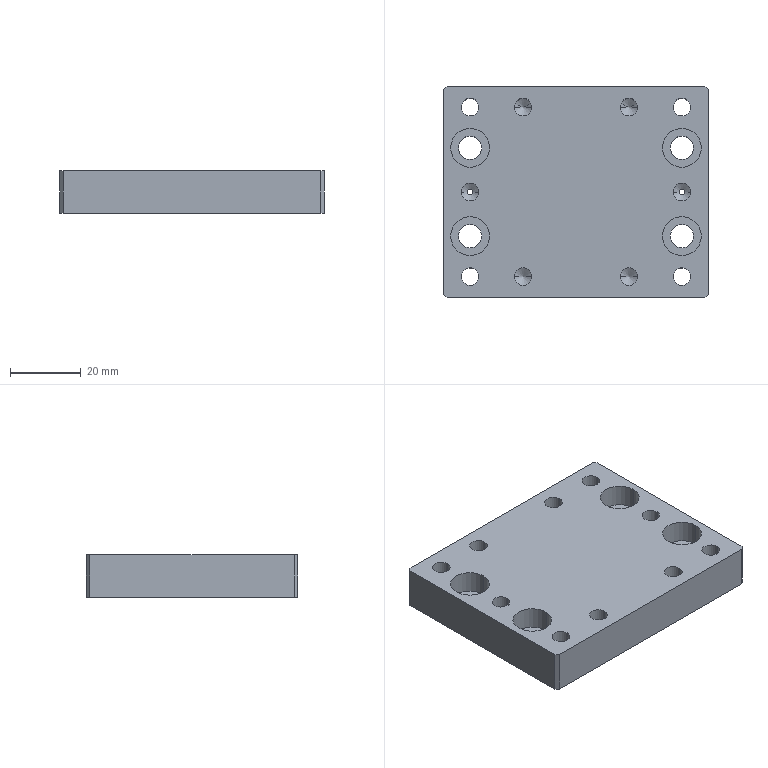Part | SolidWorks | features HoleWzd 4, Chamfer 1, Extrusion 1 | 1 solid | 62 faces | box 75 x 60 x 12 mm | volume 48559 mm3 | cylinder 36 | plane 14 | cone 12 | commonest cylinder face diameters 5 x20 6.6 x8 11 x8